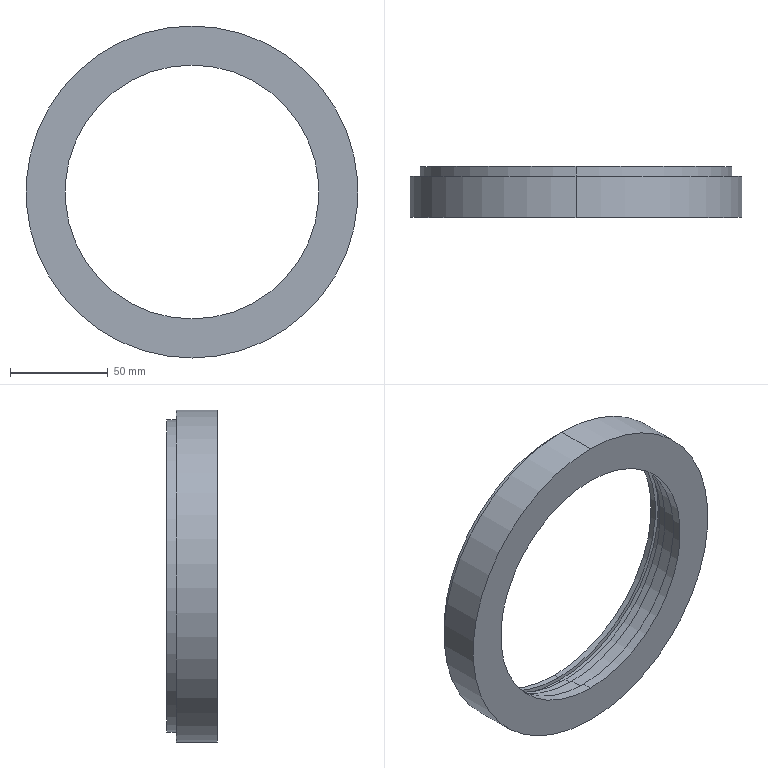Part | SolidWorks | features Revolution 1 | 1 solid | 21 faces | box 170 x 26 x 170 mm | volume 194901 mm3 | cylinder 14 | plane 7 | commonest cylinder face diameters 130 x2 135 x2 138 x2 140 x2 144 x2 160 x2
STEP:
#1=CARTESIAN_POINT('',(0.,-7.5,-72.));
#2=VERTEX_POINT('',#1);
#3=CARTESIAN_POINT('',(0.,-7.5,72.));
#4=VERTEX_POINT('',#3);
#5=CARTESIAN_POINT('',(0.,-7.5,0.));
#6=DIRECTION('',(0.,1.,0.));
#7=DIRECTION('',(0.,0.,1.));
#8=AXIS2_PLACEMENT_3D('',#5,#6,#7);
#9=CIRCLE('',#8,72.);
#10=EDGE_CURVE('',#2,#4,#9,.T.);
#11=ORIENTED_EDGE('',*,*,#10,.F.);
#12=CARTESIAN_POINT('',(0.,-3.,-72.));
#13=VERTEX_POINT('',#12);
#14=CARTESIAN_POINT('',(0.,0.,-72.));
#15=DIRECTION('',(0.,1.,0.));
#16=VECTOR('',#15,1000.);
#17=LINE('',#14,#16);
#18=EDGE_CURVE('',#2,#13,#17,.T.);
#19=ORIENTED_EDGE('',*,*,#18,.T.);
#20=CARTESIAN_POINT('',(0.,-3.,72.));
#21=VERTEX_POINT('',#20);
#22=CARTESIAN_POINT('',(0.,-3.,0.));
#23=DIRECTION('',(0.,1.,0.));
#24=DIRECTION('',(0.,0.,1.));
#25=AXIS2_PLACEMENT_3D('',#22,#23,#24);
#26=CIRCLE('',#25,72.);
#27=EDGE_CURVE('',#13,#21,#26,.T.);
#28=ORIENTED_EDGE('',*,*,#27,.T.);
#29=CARTESIAN_POINT('',(0.,0.,72.));
#30=DIRECTION('',(0.,1.,0.));
#31=VECTOR('',#30,1000.);
#32=LINE('',#29,#31);
#33=EDGE_CURVE('',#4,#21,#32,.T.);
#34=ORIENTED_EDGE('',*,*,#33,.F.);
#35=EDGE_LOOP('',(#11,#19,#28,#34));
#36=FACE_OUTER_BOUND('',#35,.T.);
#37=CARTESIAN_POINT('',(0.,0.,0.));
#38=DIRECTION('',(0.,1.,0.));
#39=DIRECTION('',(0.,0.,1.));
#40=AXIS2_PLACEMENT_3D('',#37,#38,#39);
#41=CYLINDRICAL_SURFACE('',#40,72.);
#42=ADVANCED_FACE('',(#36),#41,.F.);
#43=CARTESIAN_POINT('',(0.,-12.5,-69.));
#44=VERTEX_POINT('',#43);
#45=CARTESIAN_POINT('',(0.,-12.5,69.));
#46=VERTEX_POINT('',#45);
#47=CARTESIAN_POINT('',(0.,-12.5,0.));
#48=DIRECTION('',(0.,1.,0.));
#49=DIRECTION('',(0.,0.,1.));
#50=AXIS2_PLACEMENT_3D('',#47,#48,#49);
#51=CIRCLE('',#50,69.);
#52=EDGE_CURVE('',#44,#46,#51,.T.);
#53=ORIENTED_EDGE('',*,*,#52,.F.);
#54=CARTESIAN_POINT('',(0.,-7.5,-69.));
#55=VERTEX_POINT('',#54);
#56=CARTESIAN_POINT('',(0.,0.,-69.));
#57=DIRECTION('',(0.,1.,0.));
#58=VECTOR('',#57,1000.);
#59=LINE('',#56,#58);
#60=EDGE_CURVE('',#44,#55,#59,.T.);
#61=ORIENTED_EDGE('',*,*,#60,.T.);
#62=CARTESIAN_POINT('',(0.,-7.5,69.));
#63=VERTEX_POINT('',#62);
#64=CARTESIAN_POINT('',(0.,-7.5,0.));
#65=DIRECTION('',(0.,1.,0.));
#66=DIRECTION('',(0.,0.,1.));
#67=AXIS2_PLACEMENT_3D('',#64,#65,#66);
#68=CIRCLE('',#67,69.);
#69=EDGE_CURVE('',#55,#63,#68,.T.);
#70=ORIENTED_EDGE('',*,*,#69,.T.);
#71=CARTESIAN_POINT('',(0.,0.,69.));
#72=DIRECTION('',(0.,1.,0.));
#73=VECTOR('',#72,1000.);
#74=LINE('',#71,#73);
#75=EDGE_CURVE('',#46,#63,#74,.T.);
#76=ORIENTED_EDGE('',*,*,#75,.F.);
#77=EDGE_LOOP('',(#53,#61,#70,#76));
#78=FACE_OUTER_BOUND('',#77,.T.);
#79=CARTESIAN_POINT('',(0.,0.,0.));
#80=DIRECTION('',(0.,1.,0.));
#81=DIRECTION('',(0.,0.,1.));
#82=AXIS2_PLACEMENT_3D('',#79,#80,#81);
#83=CYLINDRICAL_SURFACE('',#82,69.);
#84=ADVANCED_FACE('',(#78),#83,.F.);
#85=CARTESIAN_POINT('',(0.,-21.,-67.5));
#86=VERTEX_POINT('',#85);
#87=CARTESIAN_POINT('',(0.,-21.,67.5));
#88=VERTEX_POINT('',#87);
#89=CARTESIAN_POINT('',(0.,-21.,0.));
#90=DIRECTION('',(0.,1.,0.));
#91=DIRECTION('',(0.,0.,1.));
#92=AXIS2_PLACEMENT_3D('',#89,#90,#91);
#93=CIRCLE('',#92,67.5);
#94=EDGE_CURVE('',#86,#88,#93,.T.);
#95=ORIENTED_EDGE('',*,*,#94,.F.);
#96=CARTESIAN_POINT('',(0.,-12.5,-67.5));
#97=VERTEX_POINT('',#96);
#98=CARTESIAN_POINT('',(0.,0.,-67.5));
#99=DIRECTION('',(0.,1.,0.));
#100=VECTOR('',#99,1000.);
#101=LINE('',#98,#100);
#102=EDGE_CURVE('',#86,#97,#101,.T.);
#103=ORIENTED_EDGE('',*,*,#102,.T.);
#104=CARTESIAN_POINT('',(0.,-12.5,67.5));
#105=VERTEX_POINT('',#104);
#106=CARTESIAN_POINT('',(0.,-12.5,0.));
#107=DIRECTION('',(0.,1.,0.));
#108=DIRECTION('',(0.,0.,1.));
#109=AXIS2_PLACEMENT_3D('',#106,#107,#108);
#110=CIRCLE('',#109,67.5);
#111=EDGE_CURVE('',#97,#105,#110,.T.);
#112=ORIENTED_EDGE('',*,*,#111,.T.);
#113=CARTESIAN_POINT('',(0.,0.,67.5));
#114=DIRECTION('',(0.,1.,0.));
#115=VECTOR('',#114,1000.);
#116=LINE('',#113,#115);
#117=EDGE_CURVE('',#88,#105,#116,.T.);
#118=ORIENTED_EDGE('',*,*,#117,.F.);
#119=EDGE_LOOP('',(#95,#103,#112,#118));
#120=FACE_OUTER_BOUND('',#119,.T.);
#121=CARTESIAN_POINT('',(0.,0.,0.));
#122=DIRECTION('',(0.,1.,0.));
#123=DIRECTION('',(0.,0.,1.));
#124=AXIS2_PLACEMENT_3D('',#121,#122,#123);
#125=CYLINDRICAL_SURFACE('',#124,67.5);
#126=ADVANCED_FACE('',(#120),#125,.F.);
#127=CARTESIAN_POINT('',(0.,-26.,-65.));
#128=VERTEX_POINT('',#127);
#129=CARTESIAN_POINT('',(0.,-26.,65.));
#130=VERTEX_POINT('',#129);
#131=CARTESIAN_POINT('',(0.,-26.,0.));
#132=DIRECTION('',(0.,1.,0.));
#133=DIRECTION('',(0.,0.,1.));
#134=AXIS2_PLACEMENT_3D('',#131,#132,#133);
#135=CIRCLE('',#134,65.);
#136=EDGE_CURVE('',#128,#130,#135,.T.);
#137=ORIENTED_EDGE('',*,*,#136,.F.);
#138=CARTESIAN_POINT('',(0.,-21.,-65.));
#139=VERTEX_POINT('',#138);
#140=CARTESIAN_POINT('',(0.,0.,-65.));
#141=DIRECTION('',(0.,1.,0.));
#142=VECTOR('',#141,1000.);
#143=LINE('',#140,#142);
#144=EDGE_CURVE('',#128,#139,#143,.T.);
#145=ORIENTED_EDGE('',*,*,#144,.T.);
#146=CARTESIAN_POINT('',(0.,-21.,65.));
#147=VERTEX_POINT('',#146);
#148=CARTESIAN_POINT('',(0.,-21.,0.));
#149=DIRECTION('',(0.,1.,0.));
#150=DIRECTION('',(0.,0.,1.));
#151=AXIS2_PLACEMENT_3D('',#148,#149,#150);
#152=CIRCLE('',#151,65.);
#153=EDGE_CURVE('',#139,#147,#152,.T.);
#154=ORIENTED_EDGE('',*,*,#153,.T.);
#155=CARTESIAN_POINT('',(0.,0.,65.));
#156=DIRECTION('',(0.,1.,0.));
#157=VECTOR('',#156,1000.);
#158=LINE('',#155,#157);
#159=EDGE_CURVE('',#130,#147,#158,.T.);
#160=ORIENTED_EDGE('',*,*,#159,.F.);
#161=EDGE_LOOP('',(#137,#145,#154,#160));
#162=FACE_OUTER_BOUND('',#161,.T.);
#163=CARTESIAN_POINT('',(0.,0.,0.));
#164=DIRECTION('',(0.,1.,0.));
#165=DIRECTION('',(0.,0.,1.));
#166=AXIS2_PLACEMENT_3D('',#163,#164,#165);
#167=CYLINDRICAL_SURFACE('',#166,65.);
#168=ADVANCED_FACE('',(#162),#167,.F.);
#169=CARTESIAN_POINT('',(0.,-26.,85.));
#170=VERTEX_POINT('',#169);
#171=CARTESIAN_POINT('',(0.,-26.,-85.));
#172=VERTEX_POINT('',#171);
#173=CARTESIAN_POINT('',(0.,-26.,0.));
#174=DIRECTION('',(0.,1.,0.));
#175=DIRECTION('',(0.,0.,1.));
#176=AXIS2_PLACEMENT_3D('',#173,#174,#175);
#177=CIRCLE('',#176,85.);
#178=EDGE_CURVE('',#170,#172,#177,.T.);
#179=ORIENTED_EDGE('',*,*,#178,.T.);
#180=CARTESIAN_POINT('',(0.,-5.,-85.));
#181=VERTEX_POINT('',#180);
#182=CARTESIAN_POINT('',(0.,0.,-85.));
#183=DIRECTION('',(0.,1.,0.));
#184=VECTOR('',#183,1000.);
#185=LINE('',#182,#184);
#186=EDGE_CURVE('',#172,#181,#185,.T.);
#187=ORIENTED_EDGE('',*,*,#186,.T.);
#188=CARTESIAN_POINT('',(0.,-5.,85.));
#189=VERTEX_POINT('',#188);
#190=CARTESIAN_POINT('',(0.,-5.,0.));
#191=DIRECTION('',(0.,1.,0.));
#192=DIRECTION('',(0.,0.,1.));
#193=AXIS2_PLACEMENT_3D('',#190,#191,#192);
#194=CIRCLE('',#193,85.);
#195=EDGE_CURVE('',#189,#181,#194,.T.);
#196=ORIENTED_EDGE('',*,*,#195,.F.);
#197=CARTESIAN_POINT('',(0.,0.,85.));
#198=DIRECTION('',(0.,1.,0.));
#199=VECTOR('',#198,1000.);
#200=LINE('',#197,#199);
#201=EDGE_CURVE('',#170,#189,#200,.T.);
#202=ORIENTED_EDGE('',*,*,#201,.F.);
#203=EDGE_LOOP('',(#179,#187,#196,#202));
#204=FACE_OUTER_BOUND('',#203,.T.);
#205=CARTESIAN_POINT('',(0.,0.,0.));
#206=DIRECTION('',(0.,1.,0.));
#207=DIRECTION('',(0.,0.,1.));
#208=AXIS2_PLACEMENT_3D('',#205,#206,#207);
#209=CYLINDRICAL_SURFACE('',#208,85.);
#210=ADVANCED_FACE('',(#204),#209,.T.);
#211=CARTESIAN_POINT('',(0.,-5.,80.));
#212=VERTEX_POINT('',#211);
#213=CARTESIAN_POINT('',(0.,-5.,-80.));
#214=VERTEX_POINT('',#213);
#215=CARTESIAN_POINT('',(0.,-5.,0.));
#216=DIRECTION('',(0.,1.,0.));
#217=DIRECTION('',(0.,0.,1.));
#218=AXIS2_PLACEMENT_3D('',#215,#216,#217);
#219=CIRCLE('',#218,80.);
#220=EDGE_CURVE('',#212,#214,#219,.T.);
#221=ORIENTED_EDGE('',*,*,#220,.T.);
#222=CARTESIAN_POINT('',(0.,0.,-80.));
#223=VERTEX_POINT('',#222);
#224=CARTESIAN_POINT('',(0.,0.,-80.));
#225=DIRECTION('',(0.,1.,0.));
#226=VECTOR('',#225,1000.);
#227=LINE('',#224,#226);
#228=EDGE_CURVE('',#214,#223,#227,.T.);
#229=ORIENTED_EDGE('',*,*,#228,.T.);
#230=CARTESIAN_POINT('',(0.,0.,80.));
#231=VERTEX_POINT('',#230);
#232=CARTESIAN_POINT('',(0.,0.,0.));
#233=DIRECTION('',(0.,1.,0.));
#234=DIRECTION('',(0.,0.,1.));
#235=AXIS2_PLACEMENT_3D('',#232,#233,#234);
#236=CIRCLE('',#235,80.);
#237=EDGE_CURVE('',#231,#223,#236,.T.);
#238=ORIENTED_EDGE('',*,*,#237,.F.);
#239=CARTESIAN_POINT('',(0.,0.,80.));
#240=DIRECTION('',(0.,1.,0.));
#241=VECTOR('',#240,1000.);
#242=LINE('',#239,#241);
#243=EDGE_CURVE('',#212,#231,#242,.T.);
#244=ORIENTED_EDGE('',*,*,#243,.F.);
#245=EDGE_LOOP('',(#221,#229,#238,#244));
#246=FACE_OUTER_BOUND('',#245,.T.);
#247=CARTESIAN_POINT('',(0.,0.,0.));
#248=DIRECTION('',(0.,1.,0.));
#249=DIRECTION('',(0.,0.,1.));
#250=AXIS2_PLACEMENT_3D('',#247,#248,#249);
#251=CYLINDRICAL_SURFACE('',#250,80.);
#252=ADVANCED_FACE('',(#246),#251,.T.);
#253=CARTESIAN_POINT('',(0.,-3.,-70.));
#254=VERTEX_POINT('',#253);
#255=CARTESIAN_POINT('',(0.,-3.,70.));
#256=VERTEX_POINT('',#255);
#257=CARTESIAN_POINT('',(0.,-3.,0.));
#258=DIRECTION('',(0.,1.,0.));
#259=DIRECTION('',(0.,0.,1.));
#260=AXIS2_PLACEMENT_3D('',#257,#258,#259);
#261=CIRCLE('',#260,70.);
#262=EDGE_CURVE('',#254,#256,#261,.T.);
#263=ORIENTED_EDGE('',*,*,#262,.F.);
#264=CARTESIAN_POINT('',(0.,0.,-70.));
#265=VERTEX_POINT('',#264);
#266=CARTESIAN_POINT('',(0.,0.,-70.));
#267=DIRECTION('',(0.,1.,0.));
#268=VECTOR('',#267,1000.);
#269=LINE('',#266,#268);
#270=EDGE_CURVE('',#254,#265,#269,.T.);
#271=ORIENTED_EDGE('',*,*,#270,.T.);
#272=CARTESIAN_POINT('',(0.,0.,70.));
#273=VERTEX_POINT('',#272);
#274=CARTESIAN_POINT('',(0.,0.,0.));
#275=DIRECTION('',(0.,1.,0.));
#276=DIRECTION('',(0.,0.,1.));
#277=AXIS2_PLACEMENT_3D('',#274,#275,#276);
#278=CIRCLE('',#277,70.);
#279=EDGE_CURVE('',#265,#273,#278,.T.);
#280=ORIENTED_EDGE('',*,*,#279,.T.);
#281=CARTESIAN_POINT('',(0.,0.,70.));
#282=DIRECTION('',(0.,1.,0.));
#283=VECTOR('',#282,1000.);
#284=LINE('',#281,#283);
#285=EDGE_CURVE('',#256,#273,#284,.T.);
#286=ORIENTED_EDGE('',*,*,#285,.F.);
#287=EDGE_LOOP('',(#263,#271,#280,#286));
#288=FACE_OUTER_BOUND('',#287,.T.);
#289=CARTESIAN_POINT('',(0.,0.,0.));
#290=DIRECTION('',(0.,1.,0.));
#291=DIRECTION('',(0.,0.,1.));
#292=AXIS2_PLACEMENT_3D('',#289,#290,#291);
#293=CYLINDRICAL_SURFACE('',#292,70.);
#294=ADVANCED_FACE('',(#288),#293,.F.);
#295=ORIENTED_EDGE('',*,*,#270,.F.);
#296=CARTESIAN_POINT('',(0.,-3.,0.));
#297=DIRECTION('',(0.,1.,0.));
#298=DIRECTION('',(0.,0.,1.));
#299=AXIS2_PLACEMENT_3D('',#296,#297,#298);
#300=CIRCLE('',#299,70.);
#301=EDGE_CURVE('',#256,#254,#300,.T.);
#302=ORIENTED_EDGE('',*,*,#301,.F.);
#303=ORIENTED_EDGE('',*,*,#285,.T.);
#304=CARTESIAN_POINT('',(0.,0.,0.));
#305=DIRECTION('',(0.,1.,0.));
#306=DIRECTION('',(0.,0.,1.));
#307=AXIS2_PLACEMENT_3D('',#304,#305,#306);
#308=CIRCLE('',#307,70.);
#309=EDGE_CURVE('',#273,#265,#308,.T.);
#310=ORIENTED_EDGE('',*,*,#309,.T.);
#311=EDGE_LOOP('',(#295,#302,#303,#310));
#312=FACE_OUTER_BOUND('',#311,.T.);
#313=CARTESIAN_POINT('',(0.,0.,0.));
#314=DIRECTION('',(0.,1.,0.));
#315=DIRECTION('',(0.,0.,1.));
#316=AXIS2_PLACEMENT_3D('',#313,#314,#315);
#317=CYLINDRICAL_SURFACE('',#316,70.);
#318=ADVANCED_FACE('',(#312),#317,.F.);
#319=ORIENTED_EDGE('',*,*,#309,.F.);
#320=ORIENTED_EDGE('',*,*,#279,.F.);
#321=EDGE_LOOP('',(#319,#320));
#322=FACE_BOUND('',#321,.T.);
#323=ORIENTED_EDGE('',*,*,#237,.T.);
#324=CARTESIAN_POINT('',(0.,0.,0.));
#325=DIRECTION('',(0.,1.,0.));
#326=DIRECTION('',(0.,0.,1.));
#327=AXIS2_PLACEMENT_3D('',#324,#325,#326);
#328=CIRCLE('',#327,80.);
#329=EDGE_CURVE('',#223,#231,#328,.T.);
#330=ORIENTED_EDGE('',*,*,#329,.T.);
#331=EDGE_LOOP('',(#323,#330));
#332=FACE_OUTER_BOUND('',#331,.T.);
#333=CARTESIAN_POINT('',(70.,0.,0.));
#334=DIRECTION('',(0.,-1.,0.));
#335=DIRECTION('',(0.,0.,-1.));
#336=AXIS2_PLACEMENT_3D('',#333,#334,#335);
#337=PLANE('',#336);
#338=ADVANCED_FACE('',(#322,#332),#337,.F.);
#339=ORIENTED_EDGE('',*,*,#228,.F.);
#340=CARTESIAN_POINT('',(0.,-5.,0.));
#341=DIRECTION('',(0.,1.,0.));
#342=DIRECTION('',(0.,0.,1.));
#343=AXIS2_PLACEMENT_3D('',#340,#341,#342);
#344=CIRCLE('',#343,80.);
#345=EDGE_CURVE('',#214,#212,#344,.T.);
#346=ORIENTED_EDGE('',*,*,#345,.T.);
#347=ORIENTED_EDGE('',*,*,#243,.T.);
#348=ORIENTED_EDGE('',*,*,#329,.F.);
#349=EDGE_LOOP('',(#339,#346,#347,#348));
#350=FACE_OUTER_BOUND('',#349,.T.);
#351=CARTESIAN_POINT('',(0.,0.,0.));
#352=DIRECTION('',(0.,1.,0.));
#353=DIRECTION('',(0.,0.,1.));
#354=AXIS2_PLACEMENT_3D('',#351,#352,#353);
#355=CYLINDRICAL_SURFACE('',#354,80.);
#356=ADVANCED_FACE('',(#350),#355,.T.);
#357=ORIENTED_EDGE('',*,*,#220,.F.);
#358=ORIENTED_EDGE('',*,*,#345,.F.);
#359=EDGE_LOOP('',(#357,#358));
#360=FACE_BOUND('',#359,.T.);
#361=ORIENTED_EDGE('',*,*,#195,.T.);
#362=CARTESIAN_POINT('',(0.,-5.,0.));
#363=DIRECTION('',(0.,1.,0.));
#364=DIRECTION('',(0.,0.,1.));
#365=AXIS2_PLACEMENT_3D('',#362,#363,#364);
#366=CIRCLE('',#365,85.);
#367=EDGE_CURVE('',#181,#189,#366,.T.);
#368=ORIENTED_EDGE('',*,*,#367,.T.);
#369=EDGE_LOOP('',(#361,#368));
#370=FACE_OUTER_BOUND('',#369,.T.);
#371=CARTESIAN_POINT('',(80.,-5.,0.));
#372=DIRECTION('',(0.,-1.,0.));
#373=DIRECTION('',(0.,0.,-1.));
#374=AXIS2_PLACEMENT_3D('',#371,#372,#373);
#375=PLANE('',#374);
#376=ADVANCED_FACE('',(#360,#370),#375,.F.);
#377=ORIENTED_EDGE('',*,*,#186,.F.);
#378=CARTESIAN_POINT('',(0.,-26.,0.));
#379=DIRECTION('',(0.,1.,0.));
#380=DIRECTION('',(0.,0.,1.));
#381=AXIS2_PLACEMENT_3D('',#378,#379,#380);
#382=CIRCLE('',#381,85.);
#383=EDGE_CURVE('',#172,#170,#382,.T.);
#384=ORIENTED_EDGE('',*,*,#383,.T.);
#385=ORIENTED_EDGE('',*,*,#201,.T.);
#386=ORIENTED_EDGE('',*,*,#367,.F.);
#387=EDGE_LOOP('',(#377,#384,#385,#386));
#388=FACE_OUTER_BOUND('',#387,.T.);
#389=CARTESIAN_POINT('',(0.,0.,0.));
#390=DIRECTION('',(0.,1.,0.));
#391=DIRECTION('',(0.,0.,1.));
#392=AXIS2_PLACEMENT_3D('',#389,#390,#391);
#393=CYLINDRICAL_SURFACE('',#392,85.);
#394=ADVANCED_FACE('',(#388),#393,.T.);
#395=ORIENTED_EDGE('',*,*,#178,.F.);
#396=ORIENTED_EDGE('',*,*,#383,.F.);
#397=EDGE_LOOP('',(#395,#396));
#398=FACE_OUTER_BOUND('',#397,.T.);
#399=CARTESIAN_POINT('',(0.,-26.,0.));
#400=DIRECTION('',(0.,1.,0.));
#401=DIRECTION('',(0.,0.,1.));
#402=AXIS2_PLACEMENT_3D('',#399,#400,#401);
#403=CIRCLE('',#402,65.);
#404=EDGE_CURVE('',#130,#128,#403,.T.);
#405=ORIENTED_EDGE('',*,*,#404,.T.);
#406=ORIENTED_EDGE('',*,*,#136,.T.);
#407=EDGE_LOOP('',(#405,#406));
#408=FACE_BOUND('',#407,.T.);
#409=CARTESIAN_POINT('',(85.,-26.,0.));
#410=DIRECTION('',(0.,1.,0.));
#411=DIRECTION('',(0.,0.,1.));
#412=AXIS2_PLACEMENT_3D('',#409,#410,#411);
#413=PLANE('',#412);
#414=ADVANCED_FACE('',(#398,#408),#413,.F.);
#415=ORIENTED_EDGE('',*,*,#144,.F.);
#416=ORIENTED_EDGE('',*,*,#404,.F.);
#417=ORIENTED_EDGE('',*,*,#159,.T.);
#418=CARTESIAN_POINT('',(0.,-21.,0.));
#419=DIRECTION('',(0.,1.,0.));
#420=DIRECTION('',(0.,0.,1.));
#421=AXIS2_PLACEMENT_3D('',#418,#419,#420);
#422=CIRCLE('',#421,65.);
#423=EDGE_CURVE('',#147,#139,#422,.T.);
#424=ORIENTED_EDGE('',*,*,#423,.T.);
#425=EDGE_LOOP('',(#415,#416,#417,#424));
#426=FACE_OUTER_BOUND('',#425,.T.);
#427=CARTESIAN_POINT('',(0.,0.,0.));
#428=DIRECTION('',(0.,1.,0.));
#429=DIRECTION('',(0.,0.,1.));
#430=AXIS2_PLACEMENT_3D('',#427,#428,#429);
#431=CYLINDRICAL_SURFACE('',#430,65.);
#432=ADVANCED_FACE('',(#426),#431,.F.);
#433=ORIENTED_EDGE('',*,*,#423,.F.);
#434=ORIENTED_EDGE('',*,*,#153,.F.);
#435=EDGE_LOOP('',(#433,#434));
#436=FACE_BOUND('',#435,.T.);
#437=CARTESIAN_POINT('',(0.,-21.,0.));
#438=DIRECTION('',(0.,1.,0.));
#439=DIRECTION('',(0.,0.,1.));
#440=AXIS2_PLACEMENT_3D('',#437,#438,#439);
#441=CIRCLE('',#440,67.5);
#442=EDGE_CURVE('',#88,#86,#441,.T.);
#443=ORIENTED_EDGE('',*,*,#442,.T.);
#444=ORIENTED_EDGE('',*,*,#94,.T.);
#445=EDGE_LOOP('',(#443,#444));
#446=FACE_OUTER_BOUND('',#445,.T.);
#447=CARTESIAN_POINT('',(65.,-21.,0.));
#448=DIRECTION('',(0.,-1.,0.));
#449=DIRECTION('',(0.,0.,-1.));
#450=AXIS2_PLACEMENT_3D('',#447,#448,#449);
#451=PLANE('',#450);
#452=ADVANCED_FACE('',(#436,#446),#451,.F.);
#453=ORIENTED_EDGE('',*,*,#102,.F.);
#454=ORIENTED_EDGE('',*,*,#442,.F.);
#455=ORIENTED_EDGE('',*,*,#117,.T.);
#456=CARTESIAN_POINT('',(0.,-12.5,0.));
#457=DIRECTION('',(0.,1.,0.));
#458=DIRECTION('',(0.,0.,1.));
#459=AXIS2_PLACEMENT_3D('',#456,#457,#458);
#460=CIRCLE('',#459,67.5);
#461=EDGE_CURVE('',#105,#97,#460,.T.);
#462=ORIENTED_EDGE('',*,*,#461,.T.);
#463=EDGE_LOOP('',(#453,#454,#455,#462));
#464=FACE_OUTER_BOUND('',#463,.T.);
#465=CARTESIAN_POINT('',(0.,0.,0.));
#466=DIRECTION('',(0.,1.,0.));
#467=DIRECTION('',(0.,0.,1.));
#468=AXIS2_PLACEMENT_3D('',#465,#466,#467);
#469=CYLINDRICAL_SURFACE('',#468,67.5);
#470=ADVANCED_FACE('',(#464),#469,.F.);
#471=ORIENTED_EDGE('',*,*,#461,.F.);
#472=ORIENTED_EDGE('',*,*,#111,.F.);
#473=EDGE_LOOP('',(#471,#472));
#474=FACE_BOUND('',#473,.T.);
#475=CARTESIAN_POINT('',(0.,-12.5,0.));
#476=DIRECTION('',(0.,1.,0.));
#477=DIRECTION('',(0.,0.,1.));
#478=AXIS2_PLACEMENT_3D('',#475,#476,#477);
#479=CIRCLE('',#478,69.);
#480=EDGE_CURVE('',#46,#44,#479,.T.);
#481=ORIENTED_EDGE('',*,*,#480,.T.);
#482=ORIENTED_EDGE('',*,*,#52,.T.);
#483=EDGE_LOOP('',(#481,#482));
#484=FACE_OUTER_BOUND('',#483,.T.);
#485=CARTESIAN_POINT('',(69.,-12.5,0.));
#486=DIRECTION('',(0.,-1.,0.));
#487=DIRECTION('',(0.,0.,-1.));
#488=AXIS2_PLACEMENT_3D('',#485,#486,#487);
#489=PLANE('',#488);
#490=ADVANCED_FACE('',(#474,#484),#489,.F.);
#491=ORIENTED_EDGE('',*,*,#60,.F.);
#492=ORIENTED_EDGE('',*,*,#480,.F.);
#493=ORIENTED_EDGE('',*,*,#75,.T.);
#494=CARTESIAN_POINT('',(0.,-7.5,0.));
#495=DIRECTION('',(0.,1.,0.));
#496=DIRECTION('',(0.,0.,1.));
#497=AXIS2_PLACEMENT_3D('',#494,#495,#496);
#498=CIRCLE('',#497,69.);
#499=EDGE_CURVE('',#63,#55,#498,.T.);
#500=ORIENTED_EDGE('',*,*,#499,.T.);
#501=EDGE_LOOP('',(#491,#492,#493,#500));
#502=FACE_OUTER_BOUND('',#501,.T.);
#503=CARTESIAN_POINT('',(0.,0.,0.));
#504=DIRECTION('',(0.,1.,0.));
#505=DIRECTION('',(0.,0.,1.));
#506=AXIS2_PLACEMENT_3D('',#503,#504,#505);
#507=CYLINDRICAL_SURFACE('',#506,69.);
#508=ADVANCED_FACE('',(#502),#507,.F.);
#509=ORIENTED_EDGE('',*,*,#499,.F.);
#510=ORIENTED_EDGE('',*,*,#69,.F.);
#511=EDGE_LOOP('',(#509,#510));
#512=FACE_BOUND('',#511,.T.);
#513=CARTESIAN_POINT('',(0.,-7.5,0.));
#514=DIRECTION('',(0.,1.,0.));
#515=DIRECTION('',(0.,0.,1.));
#516=AXIS2_PLACEMENT_3D('',#513,#514,#515);
#517=CIRCLE('',#516,72.);
#518=EDGE_CURVE('',#4,#2,#517,.T.);
#519=ORIENTED_EDGE('',*,*,#518,.T.);
#520=ORIENTED_EDGE('',*,*,#10,.T.);
#521=EDGE_LOOP('',(#519,#520));
#522=FACE_OUTER_BOUND('',#521,.T.);
#523=CARTESIAN_POINT('',(69.,-7.5,0.));
#524=DIRECTION('',(0.,-1.,0.));
#525=DIRECTION('',(0.,0.,-1.));
#526=AXIS2_PLACEMENT_3D('',#523,#524,#525);
#527=PLANE('',#526);
#528=ADVANCED_FACE('',(#512,#522),#527,.F.);
#529=ORIENTED_EDGE('',*,*,#18,.F.);
#530=ORIENTED_EDGE('',*,*,#518,.F.);
#531=ORIENTED_EDGE('',*,*,#33,.T.);
#532=CARTESIAN_POINT('',(0.,-3.,0.));
#533=DIRECTION('',(0.,1.,0.));
#534=DIRECTION('',(0.,0.,1.));
#535=AXIS2_PLACEMENT_3D('',#532,#533,#534);
#536=CIRCLE('',#535,72.);
#537=EDGE_CURVE('',#21,#13,#536,.T.);
#538=ORIENTED_EDGE('',*,*,#537,.T.);
#539=EDGE_LOOP('',(#529,#530,#531,#538));
#540=FACE_OUTER_BOUND('',#539,.T.);
#541=CARTESIAN_POINT('',(0.,0.,0.));
#542=DIRECTION('',(0.,1.,0.));
#543=DIRECTION('',(0.,0.,1.));
#544=AXIS2_PLACEMENT_3D('',#541,#542,#543);
#545=CYLINDRICAL_SURFACE('',#544,72.);
#546=ADVANCED_FACE('',(#540),#545,.F.);
#547=ORIENTED_EDGE('',*,*,#537,.F.);
#548=ORIENTED_EDGE('',*,*,#27,.F.);
#549=EDGE_LOOP('',(#547,#548));
#550=FACE_OUTER_BOUND('',#549,.T.);
#551=ORIENTED_EDGE('',*,*,#301,.T.);
#552=ORIENTED_EDGE('',*,*,#262,.T.);
#553=EDGE_LOOP('',(#551,#552));
#554=FACE_BOUND('',#553,.T.);
#555=CARTESIAN_POINT('',(72.,-3.,0.));
#556=DIRECTION('',(0.,1.,0.));
#557=DIRECTION('',(0.,0.,1.));
#558=AXIS2_PLACEMENT_3D('',#555,#556,#557);
#559=PLANE('',#558);
#560=ADVANCED_FACE('',(#550,#554),#559,.F.);
#561=CLOSED_SHELL('',(#42,#84,#126,#168,#210,#252,#294,#318,#338,#356,#376,#394,#414,#432,#452,#470,#490,#508,#528,#546,#560));
#562=MANIFOLD_SOLID_BREP('',#561);
#563=CARTESIAN_POINT('',(0.,0.,0.));
#564=DIRECTION('',(0.,0.,1.));
#565=DIRECTION('',(1.,0.,0.));
#566=AXIS2_PLACEMENT_3D('',#563,#564,#565);
#567=(LENGTH_UNIT()NAMED_UNIT(*)SI_UNIT(.MILLI.,.METRE.));
#568=UNCERTAINTY_MEASURE_WITH_UNIT(LENGTH_MEASURE(0.00001),#567,'','');
#569=(NAMED_UNIT(*)PLANE_ANGLE_UNIT()SI_UNIT($,.RADIAN.));
#570=(NAMED_UNIT(*)SI_UNIT($,.STERADIAN.)SOLID_ANGLE_UNIT());
#571=(GEOMETRIC_REPRESENTATION_CONTEXT(3)GLOBAL_UNCERTAINTY_ASSIGNED_CONTEXT((#568))GLOBAL_UNIT_ASSIGNED_CONTEXT((#567,#569,#570))REPRESENTATION_CONTEXT('',''));
#572=ADVANCED_BREP_SHAPE_REPRESENTATION('',(#562,#566),#571);